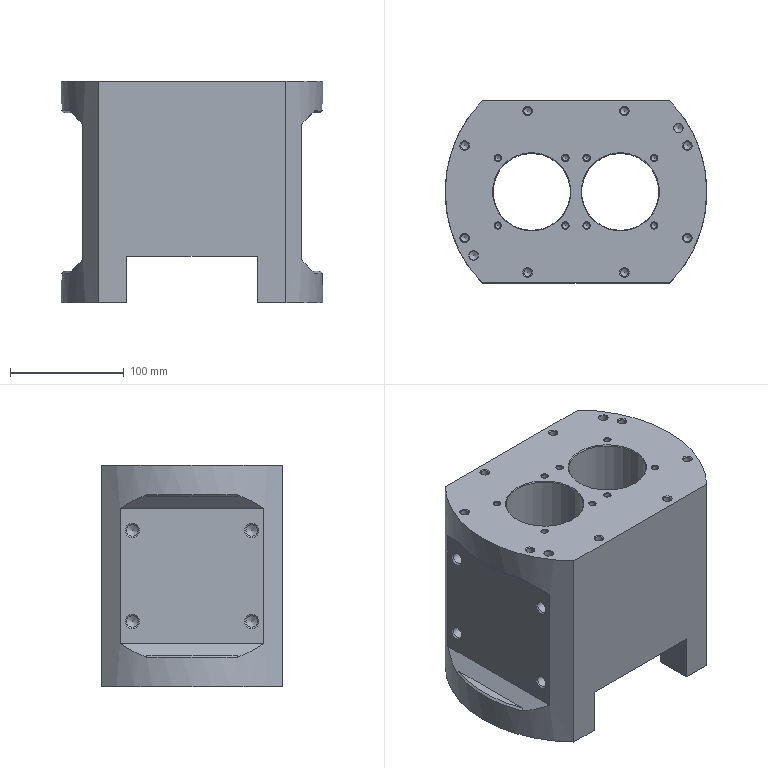NC program | NX | posted with a generic post | part box 230 x 160 x 195 mm
Lines 1 to 673 of 6533:
N10 G17 G21 G94 G90
(FLOOR_WALL_COPY_1_COPY_COPY , TOOL : D50)
N12 T02 M6
N14 G54
N16 G17 G0 G90 X-34.597 Y-36.969 B0. C0. S1200 M3
N18 G43 Z30. H2
N20 Z2.65
N22 G94 G1 Z-0.35 F1000.
N24 Y-33.969
N26 Y33.969 F2000.
N28 X0.001
N30 Y-33.969
N32 X34.6
N34 Y33.969
N36 Y36.969
N38 Z2.65
N40 G0 Z30.
N42 X-34.597 Y-40.672
N44 Z2.3
N46 G1 Z-0.7 F1000.
N48 Y-37.672
N50 Y37.672 F2000.
N52 X0.001
N54 Y-37.672
N56 X34.6
N58 Y37.672
N60 Y40.672
N62 Z2.3
N64 G0 Z30.
N66 X-34.597 Y-43.507
N68 Z1.95
N70 G1 Z-1.05 F1000.
N72 Y-40.507
N74 Y40.507 F2000.
N76 X0.001
N78 Y-40.507
N80 X34.6
N82 Y40.507
N84 Y43.507
N86 Z1.95
N88 G0 Z30.
N90 X-34.597 Y-45.891
N92 Z1.6
N94 G1 Z-1.4 F1000.
N96 Y-42.891
N98 Y42.891 F2000.
N100 X0.001
N102 Y-42.891
N104 X34.6
N106 Y42.891
N108 Y45.891
N110 Z1.6
N112 G0 Z30.
N114 X-34.597 Y-47.987
N116 Z1.25
N118 G1 Z-1.75 F1000.
N120 Y-44.987
N122 Y44.987 F2000.
N124 X0.001
N126 Y-44.987
N128 X34.6
N130 Y44.987
N132 Y47.987
N134 Z1.25
N136 G0 Z30.
N138 X-34.597 Y-49.878
N140 Z0.9
N142 G1 Z-2.1 F1000.
N144 Y-46.878
N146 Y46.878 F2000.
N148 X0.001
N150 Y-46.878
N152 X34.6
N154 Y46.878
N156 Y49.878
N158 Z0.9
N160 G0 Z30.
N162 X-34.597 Y-51.613
N164 Z0.55
N166 G1 Z-2.45 F1000.
N168 Y-48.613
N170 Y48.613 F2000.
N172 X0.001
N174 Y-48.613
N176 X34.6
N178 Y48.613
N180 Y51.613
N182 Z0.55
N184 G0 Z30.
N186 X-34.597 Y-53.223
N188 Z0.2
N190 G1 Z-2.8 F1000.
N192 Y-50.223
N194 Y50.223 F2000.
N196 X0.001
N198 Y-50.223
N200 X34.6
N202 Y50.223
N204 Y53.223
N206 Z0.2
N208 G0 Z30.
N210 X-34.597 Y-54.733
N212 Z-0.15
N214 G1 Z-3.15 F1000.
N216 Y-51.733
N218 Y51.733 F2000.
N220 X0.001
N222 Y-51.733
N224 X34.6
N226 Y51.733
N228 Y54.733
N230 Z-0.15
N232 G0 Z30.
N234 X-34.597 Y-56.157
N236 Z-0.5
N238 G1 Z-3.5 F1000.
N240 Y-53.157
N242 Y53.157 F2000.
N244 X0.001
N246 Y-53.157
N248 X34.6
N250 Y53.157
N252 Y56.157
N254 Z-0.5
N256 G0 Z30.
N258 X-34.597 Y-57.508
N260 Z-0.85
N262 G1 Z-3.85 F1000.
N264 Y-54.508
N266 Y54.508 F2000.
N268 X0.001
N270 Y-54.508
N272 X34.6
N274 Y54.508
N276 Y57.508
N278 Z-0.85
N280 G0 Z30.
N282 X-34.597 Y-58.796
N284 Z-1.2
N286 G1 Z-4.2 F1000.
N288 Y-55.796
N290 Y55.796 F2000.
N292 X0.001
N294 Y-55.796
N296 X34.6
N298 Y55.796
N300 Y58.796
N302 Z-1.2
N304 G0 Z30.
N306 X-34.597 Y-60.029
N308 Z-1.55
N310 G1 Z-4.55 F1000.
N312 Y-57.029
N314 Y57.029 F2000.
N316 X0.001
N318 Y-57.029
N320 X34.6
N322 Y57.029
N324 Y60.029
N326 Z-1.55
N328 G0 Z30.
N330 X-34.597 Y-61.212
N332 Z-1.9
N334 G1 Z-4.9 F1000.
N336 Y-58.212
N338 Y58.212 F2000.
N340 X0.001
N342 Y-58.212
N344 X34.6
N346 Y58.212
N348 Y61.212
N350 Z-1.9
N352 G0 Z30.
N354 X-34.597 Y-62.351
N356 Z-2.25
N358 G1 Z-5.25 F1000.
N360 Y-59.351
N362 Y59.351 F2000.
N364 X0.001
N366 Y-59.351
N368 X34.6
N370 Y59.351
N372 Y62.351
N374 Z-2.25
N376 G0 Z30.
N378 X-34.597 Y-63.45
N380 Z-2.6
N382 G1 Z-5.6 F1000.
N384 Y-60.45
N386 Y60.45 F2000.
N388 X0.001
N390 Y-60.45
N392 X34.6
N394 Y60.45
N396 Y63.45
N398 Z-2.6
N400 G0 Z30.
N402 X-34.597 Y-64.512
N404 Z-2.95
N406 G1 Z-5.95 F1000.
N408 Y-61.512
N410 Y61.512 F2000.
N412 X0.001
N414 Y-61.512
N416 X34.6
N418 Y61.512
N420 Y64.512
N422 Z-2.95
N424 G0 Z30.
N426 X-34.597 Y-65.541
N428 Z-3.3
N430 G1 Z-6.3 F1000.
N432 Y-62.541
N434 Y62.541 F2000.
N436 X0.001
N438 Y-62.541
N440 X34.6
N442 Y62.541
N444 Y65.541
N446 Z-3.3
N448 G0 Z30.
N450 X-34.597 Y-66.54
N452 Z-3.65
N454 G1 Z-6.65 F1000.
N456 Y-63.54
N458 Y63.54 F2000.
N460 X0.001
N462 Y-63.54
N464 X34.6
N466 Y63.54
N468 Y66.54
N470 Z-3.65
N472 G0 Z30.
N474 X-34.597 Y-67.51
N476 Z-4.
N478 G1 Z-7. F1000.
N480 Y-64.51
N482 Y64.51 F2000.
N484 X0.001
N486 Y-64.51
N488 X34.6
N490 Y64.51
N492 Y67.51
N494 Z-4.
N496 G0 Z30.
N498 X-34.597 Y-68.454
N500 Z-4.35
N502 G1 Z-7.35 F1000.
N504 Y-65.454
N506 Y65.454 F2000.
N508 X0.001
N510 Y-65.454
N512 X34.6
N514 Y65.454
N516 Y68.454
N518 Z-4.35
N520 G0 Z30.
N522 X-34.597 Y-69.373
N524 Z-4.7
N526 G1 Z-7.7 F1000.
N528 Y-66.373
N530 Y66.373 F2000.
N532 X0.001
N534 Y-66.373
N536 X34.6
N538 Y66.373
N540 Y69.373
N542 Z-4.7
N544 G0 Z30.
N546 X-34.597 Y-70.27
N548 Z-5.05
N550 G1 Z-8.05 F1000.
N552 Y-67.27
N554 Y67.27 F2000.
N556 X0.001
N558 Y-67.27
N560 X34.6
N562 Y67.27
N564 Y70.27
N566 Z-5.05
N568 G0 Z30.
N570 X-34.597 Y-71.145
N572 Z-5.4
N574 G1 Z-8.4 F1000.
N576 Y-68.145
N578 Y68.145 F2000.
N580 X0.001
N582 Y-68.145
N584 X34.6
N586 Y68.145
N588 Y71.145
N590 Z-5.4
N592 G0 Z30.
N594 X-34.597 Y-72.
N596 Z-5.75
N598 G1 Z-8.75 F1000.
N600 Y-69.
N602 Y69. F2000.
N604 X0.001
N606 Y-69.
N608 X34.6
N610 Y69.
N612 Y72.
N614 Z-5.75
N616 G0 Z30.
N618 X-34.597 Y-72.836
N620 Z-6.1
N622 G1 Z-9.1 F1000.
N624 Y-69.836
N626 Y69.836 F2000.
N628 X0.001
N630 Y-69.836
N632 X34.6
N634 Y69.836
N636 Y72.836
N638 Z-6.1
N640 G0 Z30.
N642 X-34.597 Y-73.653
N644 Z-6.45
N646 G1 Z-9.45 F1000.
N648 Y-70.653
N650 Y70.653 F2000.
N652 X0.001
N654 Y-70.653
N656 X34.6
N658 Y70.653
N660 Y73.653
N662 Z-6.45
N664 G0 Z30.
N666 X-34.597 Y-74.454
N668 Z-6.8
N670 G1 Z-9.8 F1000.
N672 Y-71.454
N674 Y71.454 F2000.
N676 X0.001
N678 Y-71.454
N680 X34.6
N682 Y71.454
N684 Y74.454
N686 Z-6.8
N688 G0 Z30.
N690 X-34.597 Y-75.239
N692 Z-7.15
N694 G1 Z-10.15 F1000.
N696 Y-72.239
N698 Y72.239 F2000.
N700 X0.001
N702 Y-72.239
N704 X34.6
N706 Y72.239
N708 Y75.239
N710 Z-7.15
N712 G0 Z30.
N714 X-34.597 Y-76.008
N716 Z-7.5
N718 G1 Z-10.5 F1000.
N720 Y-73.008
N722 Y73.008 F2000.
N724 X0.001
N726 Y-73.008
N728 X34.6
N730 Y73.008
N732 Y76.008
N734 Z-7.5
N736 G0 Z30.
N738 X-34.597 Y-76.763
N740 Z-7.85
N742 G1 Z-10.85 F1000.
N744 Y-73.763
N746 Y73.763 F2000.
N748 X0.001
N750 Y-73.763
N752 X34.6
N754 Y73.763
N756 Y76.763
N758 Z-7.85
N760 G0 Z30.
N762 X-34.597 Y-77.503
N764 Z-8.2
N766 G1 Z-11.2 F1000.
N768 Y-74.503
N770 Y74.503 F2000.
N772 X0.001
N774 Y-74.503
N776 X34.6
N778 Y74.503
N780 Y77.503
N782 Z-8.2
N784 G0 Z30.
N786 X-34.597 Y-78.231
N788 Z-8.55
N790 G1 Z-11.55 F1000.
N792 Y-75.231
N794 Y75.231 F2000.
N796 X0.001
N798 Y-75.231
N800 X34.6
N802 Y75.231
N804 Y78.231
N806 Z-8.55
N808 G0 Z30.
N810 X-34.597 Y-78.945
N812 Z-8.9
N814 G1 Z-11.9 F1000.
N816 Y-75.945
N818 Y75.945 F2000.
N820 X0.001
N822 Y-75.945
N824 X34.6
N826 Y75.945
N828 Y78.945
N830 Z-8.9
N832 G0 Z30.
N834 X-34.597 Y-79.647
N836 Z-9.25
N838 G1 Z-12.25 F1000.
N840 Y-76.647
N842 Y76.647 F2000.
N844 X0.001
N846 Y-76.647
N848 X34.6
N850 Y76.647
N852 Y79.647
N854 Z-9.25
N856 G0 Z30.
N858 X-34.597 Y-80.338
N860 Z-9.6
N862 G1 Z-12.6 F1000.
N864 Y-77.338
N866 Y77.338 F2000.
N868 X0.001
N870 Y-77.338
N872 X34.6
N874 Y77.338
N876 Y80.338
N878 Z-9.6
N880 G0 Z30.
N882 X-34.597 Y-81.017
N884 Z-9.95
N886 G1 Z-12.95 F1000.
N888 Y-78.017
N890 Y78.017 F2000.
N892 X0.001
N894 Y-78.017
N896 X34.6
N898 Y78.017
N900 Y81.017
N902 Z-9.95
N904 G0 Z30.
N906 X-34.597 Y-81.685
N908 Z-10.3
N910 G1 Z-13.3 F1000.
N912 Y-78.685
N914 Y78.685 F2000.
N916 X0.001
N918 Y-78.685
N920 X34.6
N922 Y78.685
N924 Y81.685
N926 Z-10.3
N928 G0 Z30.
N930 X-34.597 Y-82.343
N932 Z-10.65
N934 G1 Z-13.65 F1000.
N936 Y-79.343
N938 Y79.343 F2000.
N940 X0.001
N942 Y-79.343
N944 X34.6
N946 Y79.343
N948 Y82.343
N950 Z-10.65
N952 G0 Z30.
N954 X-34.597 Y-82.991
N956 Z-11.
N958 G1 Z-14. F1000.
N960 Y-79.991
N962 Y79.991 F2000.
N964 X0.001
N966 Y-79.991
N968 X34.6
N970 Y79.991
N972 Y82.991
N974 Z-11.
N976 G0 Z30.
N978 X-34.597 Y-83.629
N980 Z-11.35
N982 G1 Z-14.35 F1000.
N984 Y-80.629
N986 Y80.629 F2000.
N988 X0.001
N990 Y-80.629
N992 X34.6
N994 Y80.629
N996 Y83.629
N998 Z-11.35
N1000 G0 Z30.
N1002 X-34.597 Y-84.258
N1004 Z-11.7
N1006 G1 Z-14.7 F1000.
N1008 Y-81.258
N1010 Y81.258 F2000.
N1012 X0.001
N1014 Y-81.258
N1016 X34.6
N1018 Y81.258
N1020 Y84.258
N1022 Z-11.7
N1024 G0 Z30.
N1026 X-34.597 Y-84.877
N1028 Z-12.05
N1030 G1 Z-15.05 F1000.
N1032 Y-81.877
N1034 Y81.877 F2000.
N1036 X0.001
N1038 Y-81.877
N1040 X34.6
N1042 Y81.877
N1044 Y84.877
N1046 Z-12.05
N1048 G0 Z30.
N1050 X-34.597 Y-85.488
N1052 Z-12.4
N1054 G1 Z-15.4 F1000.
N1056 Y-82.488
N1058 Y82.488 F2000.
N1060 X0.001
N1062 Y-82.488
N1064 X34.6
N1066 Y82.488
N1068 Y85.488
N1070 Z-12.4
N1072 G0 Z30.
N1074 X-34.597 Y-86.09
N1076 Z-12.75
N1078 G1 Z-15.75 F1000.
N1080 Y-83.09
N1082 Y83.09 F2000.
N1084 X0.001
N1086 Y-83.09
N1088 X34.6
N1090 Y83.09
N1092 Y86.09
N1094 Z-12.75
N1096 G0 Z30.
N1098 X-34.597 Y-86.684
N1100 Z-13.1
N1102 G1 Z-16.1 F1000.
N1104 Y-83.684
N1106 Y83.684 F2000.
N1108 X0.001
N1110 Y-83.684
N1112 X34.6
N1114 Y83.684
N1116 Y86.684
N1118 Z-13.1
N1120 G0 Z30.
N1122 X-34.597 Y-87.27
N1124 Z-13.45
N1126 G1 Z-16.45 F1000.
N1128 Y-84.27
N1130 Y84.27 F2000.
N1132 X0.001
N1134 Y-84.27
N1136 X34.6
N1138 Y84.27
N1140 Y87.27
N1142 Z-13.45
N1144 G0 Z30.
N1146 X-34.597 Y-87.848
N1148 Z-13.8
N1150 G1 Z-16.8 F1000.
N1152 Y-84.848
N1154 Y84.848 F2000.
N1156 X0.001
N1158 Y-84.848
N1160 X34.6
N1162 Y84.848
N1164 Y87.848
N1166 Z-13.8
N1168 G0 Z30.
N1170 X-34.597 Y-88.418
N1172 Z-14.15
N1174 G1 Z-17.15 F1000.
N1176 Y-85.418
N1178 Y85.418 F2000.
N1180 X0.001
N1182 Y-85.418
N1184 X34.6
N1186 Y85.418
N1188 Y88.418
N1190 Z-14.15
N1192 G0 Z30.
N1194 X-34.597 Y-88.982
N1196 Z-14.5
N1198 G1 Z-17.5 F1000.
N1200 Y-85.982
N1202 Y85.982 F2000.
N1204 X0.001
N1206 Y-85.982
N1208 X34.6
N1210 Y85.982
N1212 Y88.982
N1214 Z-14.5
N1216 G0 Z30.
N1218 X-34.597 Y-89.538
N1220 Z-14.85
N1222 G1 Z-17.85 F1000.
N1224 Y-86.538
N1226 Y86.538 F2000.
N1228 X0.001
N1230 Y-86.538
N1232 X34.6
N1234 Y86.538
N1236 Y89.538
N1238 Z-14.85
N1240 G0 Z30.
N1242 X-34.597 Y-90.087
N1244 Z-15.2
N1246 G1 Z-18.2 F1000.
N1248 Y-87.087
N1250 Y87.087 F2000.
N1252 X0.001
N1254 Y-87.087
N1256 X34.6
N1258 Y87.087
N1260 Y90.087
N1262 Z-15.2
N1264 G0 Z30.
N1266 X-34.597 Y-90.629
N1268 Z-15.55
N1270 G1 Z-18.55 F1000.
N1272 Y-87.629
N1274 Y87.629 F2000.
N1276 X0.001
N1278 Y-87.629
N1280 X34.6
N1282 Y87.629
N1284 Y90.629
N1286 Z-15.55
N1288 G0 Z30.
N1290 X-34.597 Y-91.165
N1292 Z-15.9
N1294 G1 Z-18.9 F1000.
N1296 Y-88.165
N1298 Y88.165 F2000.
N1300 X0.001
N1302 Y-88.165
N1304 X34.6
N1306 Y88.165
N1308 Y91.165
N1310 Z-15.9
N1312 G0 Z30.
(FLOOR_WALL_COPY_COPY_COPY_COPY , TOOL : D50)
N1314 X-34.497 Y-91.317 S2500
N1316 Z-16.
N1318 G1 Z-19. F1000.
N1320 Y-88.317
N1322 Y88.317
N1324 X0.001
N1326 Y-88.317
N1328 X34.5
N1330 Y88.317
N1332 Y91.317
N1334 Z-16.
N1336 G0 Z30.
N1338 M5